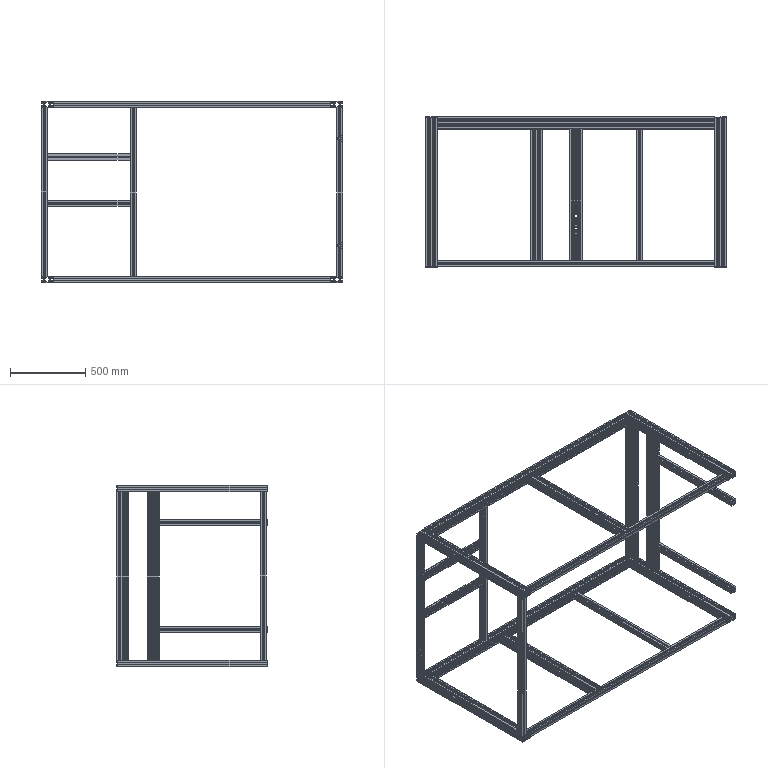Part | NX | 20 solids | 1330 faces | box 2000 x 996 x 1200 mm | volume 24167688 mm3 | plane 1148 | cylinder 182 | commonest cylinder face diameters 6 x52 8 x48 6.75 x20 19.333 x16 19.4 x16 2.5 x12